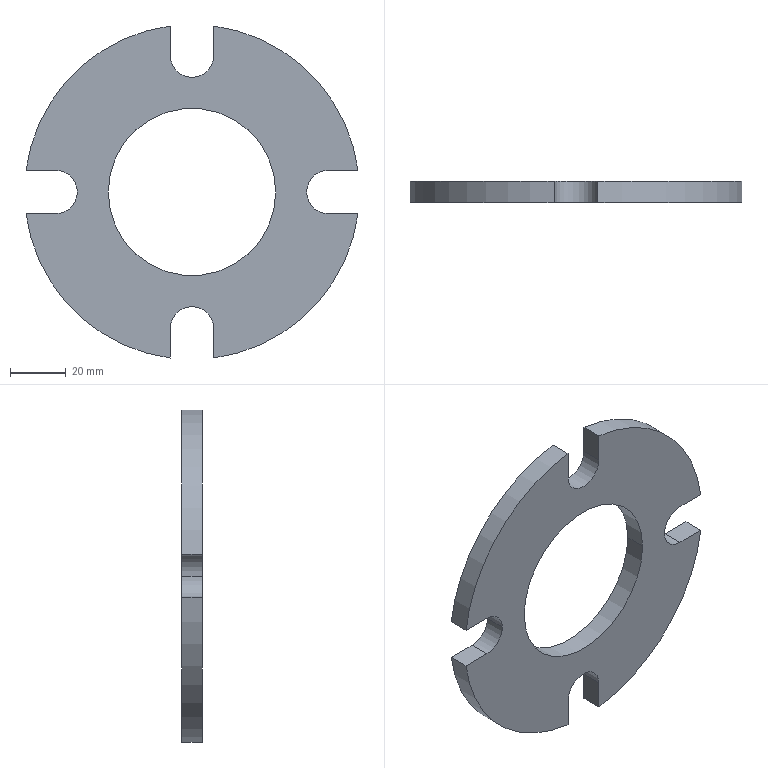Part | STEP file | Scale factor 1[14] | 1 solid | 22 faces | box 118.982 x 7.5 x 118.982 mm | volume 55635 mm3 | cylinder 12 | plane 10 | commonest cylinder face diameters 15.6 x6 120 x4 60 x2
STEP:
#1=CARTESIAN_POINT('',(-707.638,-288.773,3238.5));
#2=VERTEX_POINT('',#1);
#3=CARTESIAN_POINT('',(-699.838,-288.773,3246.3));
#4=VERTEX_POINT('',#3);
#5=CARTESIAN_POINT('',(-699.838,-288.773,3238.5));
#6=DIRECTION('',(0.,1.,0.));
#7=DIRECTION('',(1.,0.,0.000000001));
#8=AXIS2_PLACEMENT_3D('',#5,#6,#7);
#9=CIRCLE('',#8,7.8);
#10=EDGE_CURVE('',#2,#4,#9,.T.);
#11=ORIENTED_EDGE('',*,*,#10,.F.);
#12=CARTESIAN_POINT('',(-707.638,-281.273,3238.5));
#13=VERTEX_POINT('',#12);
#14=CARTESIAN_POINT('',(-707.638,-288.773,3238.5));
#15=DIRECTION('',(0.,1.,0.));
#16=VECTOR('',#15,1000.);
#17=LINE('',#14,#16);
#18=EDGE_CURVE('',#2,#13,#17,.T.);
#19=ORIENTED_EDGE('',*,*,#18,.T.);
#20=CARTESIAN_POINT('',(-699.838,-281.273,3246.3));
#21=VERTEX_POINT('',#20);
#22=CARTESIAN_POINT('',(-699.838,-281.273,3238.5));
#23=DIRECTION('',(0.,1.,0.));
#24=DIRECTION('',(1.,0.,0.000000001));
#25=AXIS2_PLACEMENT_3D('',#22,#23,#24);
#26=CIRCLE('',#25,7.8);
#27=EDGE_CURVE('',#13,#21,#26,.T.);
#28=ORIENTED_EDGE('',*,*,#27,.T.);
#29=CARTESIAN_POINT('',(-699.838,-288.773,3246.3));
#30=DIRECTION('',(0.,1.,0.));
#31=VECTOR('',#30,1000.);
#32=LINE('',#29,#31);
#33=EDGE_CURVE('',#4,#21,#32,.T.);
#34=ORIENTED_EDGE('',*,*,#33,.F.);
#35=EDGE_LOOP('',(#11,#19,#28,#34));
#36=FACE_OUTER_BOUND('',#35,.T.);
#37=CARTESIAN_POINT('',(-699.838,-288.773,3238.5));
#38=DIRECTION('',(0.,1.,0.));
#39=DIRECTION('',(-1.,0.,-0.000000001));
#40=AXIS2_PLACEMENT_3D('',#37,#38,#39);
#41=CYLINDRICAL_SURFACE('',#40,7.8);
#42=ADVANCED_FACE('',(#36),#41,.F.);
#43=CARTESIAN_POINT('',(-718.738,-281.273,3238.5));
#44=VERTEX_POINT('',#43);
#45=CARTESIAN_POINT('',(-778.738,-281.273,3238.5));
#46=VERTEX_POINT('',#45);
#47=CARTESIAN_POINT('',(-748.738,-281.273,3238.5));
#48=DIRECTION('',(0.,-1.,0.));
#49=DIRECTION('',(-1.,0.,-0.000000001));
#50=AXIS2_PLACEMENT_3D('',#47,#48,#49);
#51=CIRCLE('',#50,30.);
#52=EDGE_CURVE('',#44,#46,#51,.T.);
#53=ORIENTED_EDGE('',*,*,#52,.F.);
#54=CARTESIAN_POINT('',(-718.738,-288.773,3238.5));
#55=VERTEX_POINT('',#54);
#56=CARTESIAN_POINT('',(-718.738,-281.273,3238.5));
#57=DIRECTION('',(0.,1.,0.));
#58=VECTOR('',#57,1000.);
#59=LINE('',#56,#58);
#60=EDGE_CURVE('',#55,#44,#59,.T.);
#61=ORIENTED_EDGE('',*,*,#60,.F.);
#62=CARTESIAN_POINT('',(-778.738,-288.773,3238.5));
#63=VERTEX_POINT('',#62);
#64=CARTESIAN_POINT('',(-748.738,-288.773,3238.5));
#65=DIRECTION('',(0.,-1.,0.));
#66=DIRECTION('',(-1.,0.,-0.000000001));
#67=AXIS2_PLACEMENT_3D('',#64,#65,#66);
#68=CIRCLE('',#67,30.);
#69=EDGE_CURVE('',#55,#63,#68,.T.);
#70=ORIENTED_EDGE('',*,*,#69,.T.);
#71=CARTESIAN_POINT('',(-778.738,-281.273,3238.5));
#72=DIRECTION('',(0.,1.,0.));
#73=VECTOR('',#72,1000.);
#74=LINE('',#71,#73);
#75=EDGE_CURVE('',#63,#46,#74,.T.);
#76=ORIENTED_EDGE('',*,*,#75,.T.);
#77=EDGE_LOOP('',(#53,#61,#70,#76));
#78=FACE_OUTER_BOUND('',#77,.T.);
#79=CARTESIAN_POINT('',(-748.738,-281.273,3238.5));
#80=DIRECTION('',(0.,-1.,0.));
#81=DIRECTION('',(1.,0.,0.000000001));
#82=AXIS2_PLACEMENT_3D('',#79,#80,#81);
#83=CYLINDRICAL_SURFACE('',#82,30.);
#84=ADVANCED_FACE('',(#78),#83,.F.);
#85=CARTESIAN_POINT('',(-789.838,-288.773,3238.5));
#86=VERTEX_POINT('',#85);
#87=CARTESIAN_POINT('',(-797.638,-288.773,3230.7));
#88=VERTEX_POINT('',#87);
#89=CARTESIAN_POINT('',(-797.638,-288.773,3238.5));
#90=DIRECTION('',(0.,1.,0.));
#91=DIRECTION('',(1.,0.,0.000000001));
#92=AXIS2_PLACEMENT_3D('',#89,#90,#91);
#93=CIRCLE('',#92,7.8);
#94=EDGE_CURVE('',#86,#88,#93,.T.);
#95=ORIENTED_EDGE('',*,*,#94,.F.);
#96=CARTESIAN_POINT('',(-789.838,-281.273,3238.5));
#97=VERTEX_POINT('',#96);
#98=CARTESIAN_POINT('',(-789.838,-288.773,3238.5));
#99=DIRECTION('',(0.,1.,0.));
#100=VECTOR('',#99,1000.);
#101=LINE('',#98,#100);
#102=EDGE_CURVE('',#86,#97,#101,.T.);
#103=ORIENTED_EDGE('',*,*,#102,.T.);
#104=CARTESIAN_POINT('',(-797.638,-281.273,3230.7));
#105=VERTEX_POINT('',#104);
#106=CARTESIAN_POINT('',(-797.638,-281.273,3238.5));
#107=DIRECTION('',(0.,1.,0.));
#108=DIRECTION('',(1.,0.,0.000000001));
#109=AXIS2_PLACEMENT_3D('',#106,#107,#108);
#110=CIRCLE('',#109,7.8);
#111=EDGE_CURVE('',#97,#105,#110,.T.);
#112=ORIENTED_EDGE('',*,*,#111,.T.);
#113=CARTESIAN_POINT('',(-797.638,-288.773,3230.7));
#114=DIRECTION('',(0.,1.,0.));
#115=VECTOR('',#114,1000.);
#116=LINE('',#113,#115);
#117=EDGE_CURVE('',#88,#105,#116,.T.);
#118=ORIENTED_EDGE('',*,*,#117,.F.);
#119=EDGE_LOOP('',(#95,#103,#112,#118));
#120=FACE_OUTER_BOUND('',#119,.T.);
#121=CARTESIAN_POINT('',(-797.638,-288.773,3238.5));
#122=DIRECTION('',(0.,1.,0.));
#123=DIRECTION('',(-1.,0.,-0.000000001));
#124=AXIS2_PLACEMENT_3D('',#121,#122,#123);
#125=CYLINDRICAL_SURFACE('',#124,7.8);
#126=ADVANCED_FACE('',(#120),#125,.F.);
#127=CARTESIAN_POINT('',(-808.229,-288.773,3246.3));
#128=VERTEX_POINT('',#127);
#129=CARTESIAN_POINT('',(-808.229,-281.273,3246.3));
#130=VERTEX_POINT('',#129);
#131=CARTESIAN_POINT('',(-808.229,-288.773,3246.3));
#132=DIRECTION('',(0.,1.,0.));
#133=VECTOR('',#132,1000.);
#134=LINE('',#131,#133);
#135=EDGE_CURVE('',#128,#130,#134,.T.);
#136=ORIENTED_EDGE('',*,*,#135,.F.);
#137=CARTESIAN_POINT('',(-756.538,-288.773,3297.991));
#138=VERTEX_POINT('',#137);
#139=CARTESIAN_POINT('',(-748.738,-288.773,3238.5));
#140=DIRECTION('',(0.,1.,0.));
#141=DIRECTION('',(1.,0.,0.000000001));
#142=AXIS2_PLACEMENT_3D('',#139,#140,#141);
#143=CIRCLE('',#142,60.);
#144=EDGE_CURVE('',#128,#138,#143,.T.);
#145=ORIENTED_EDGE('',*,*,#144,.T.);
#146=CARTESIAN_POINT('',(-756.538,-281.273,3297.991));
#147=VERTEX_POINT('',#146);
#148=CARTESIAN_POINT('',(-756.538,-288.773,3297.991));
#149=DIRECTION('',(0.,1.,0.));
#150=VECTOR('',#149,1000.);
#151=LINE('',#148,#150);
#152=EDGE_CURVE('',#138,#147,#151,.T.);
#153=ORIENTED_EDGE('',*,*,#152,.T.);
#154=CARTESIAN_POINT('',(-748.738,-281.273,3238.5));
#155=DIRECTION('',(0.,1.,0.));
#156=DIRECTION('',(1.,0.,0.000000001));
#157=AXIS2_PLACEMENT_3D('',#154,#155,#156);
#158=CIRCLE('',#157,60.);
#159=EDGE_CURVE('',#130,#147,#158,.T.);
#160=ORIENTED_EDGE('',*,*,#159,.F.);
#161=EDGE_LOOP('',(#136,#145,#153,#160));
#162=FACE_OUTER_BOUND('',#161,.T.);
#163=CARTESIAN_POINT('',(-748.738,-281.273,3238.5));
#164=DIRECTION('',(0.,-1.,0.));
#165=DIRECTION('',(1.,0.,0.000000001));
#166=AXIS2_PLACEMENT_3D('',#163,#164,#165);
#167=CYLINDRICAL_SURFACE('',#166,60.);
#168=ADVANCED_FACE('',(#162),#167,.T.);
#169=CARTESIAN_POINT('',(-740.938,-288.773,3297.991));
#170=VERTEX_POINT('',#169);
#171=CARTESIAN_POINT('',(-740.938,-281.273,3297.991));
#172=VERTEX_POINT('',#171);
#173=CARTESIAN_POINT('',(-740.938,-288.773,3297.991));
#174=DIRECTION('',(0.,1.,0.));
#175=VECTOR('',#174,1000.);
#176=LINE('',#173,#175);
#177=EDGE_CURVE('',#170,#172,#176,.T.);
#178=ORIENTED_EDGE('',*,*,#177,.F.);
#179=CARTESIAN_POINT('',(-689.247,-288.773,3246.3));
#180=VERTEX_POINT('',#179);
#181=CARTESIAN_POINT('',(-748.738,-288.773,3238.5));
#182=DIRECTION('',(0.,1.,0.));
#183=DIRECTION('',(1.,0.,0.000000001));
#184=AXIS2_PLACEMENT_3D('',#181,#182,#183);
#185=CIRCLE('',#184,60.);
#186=EDGE_CURVE('',#170,#180,#185,.T.);
#187=ORIENTED_EDGE('',*,*,#186,.T.);
#188=CARTESIAN_POINT('',(-689.247,-281.273,3246.3));
#189=VERTEX_POINT('',#188);
#190=CARTESIAN_POINT('',(-689.247,-288.773,3246.3));
#191=DIRECTION('',(0.,1.,0.));
#192=VECTOR('',#191,1000.);
#193=LINE('',#190,#192);
#194=EDGE_CURVE('',#180,#189,#193,.T.);
#195=ORIENTED_EDGE('',*,*,#194,.T.);
#196=CARTESIAN_POINT('',(-748.738,-281.273,3238.5));
#197=DIRECTION('',(0.,1.,0.));
#198=DIRECTION('',(1.,0.,0.000000001));
#199=AXIS2_PLACEMENT_3D('',#196,#197,#198);
#200=CIRCLE('',#199,60.);
#201=EDGE_CURVE('',#172,#189,#200,.T.);
#202=ORIENTED_EDGE('',*,*,#201,.F.);
#203=EDGE_LOOP('',(#178,#187,#195,#202));
#204=FACE_OUTER_BOUND('',#203,.T.);
#205=CARTESIAN_POINT('',(-748.738,-281.273,3238.5));
#206=DIRECTION('',(0.,-1.,0.));
#207=DIRECTION('',(1.,0.,0.000000001));
#208=AXIS2_PLACEMENT_3D('',#205,#206,#207);
#209=CYLINDRICAL_SURFACE('',#208,60.);
#210=ADVANCED_FACE('',(#204),#209,.T.);
#211=CARTESIAN_POINT('',(-689.247,-288.773,3230.7));
#212=VERTEX_POINT('',#211);
#213=CARTESIAN_POINT('',(-689.247,-281.273,3230.7));
#214=VERTEX_POINT('',#213);
#215=CARTESIAN_POINT('',(-689.247,-288.773,3230.7));
#216=DIRECTION('',(0.,1.,0.));
#217=VECTOR('',#216,1000.);
#218=LINE('',#215,#217);
#219=EDGE_CURVE('',#212,#214,#218,.T.);
#220=ORIENTED_EDGE('',*,*,#219,.F.);
#221=CARTESIAN_POINT('',(-740.938,-288.773,3179.009));
#222=VERTEX_POINT('',#221);
#223=CARTESIAN_POINT('',(-748.738,-288.773,3238.5));
#224=DIRECTION('',(0.,1.,0.));
#225=DIRECTION('',(1.,0.,0.000000001));
#226=AXIS2_PLACEMENT_3D('',#223,#224,#225);
#227=CIRCLE('',#226,60.);
#228=EDGE_CURVE('',#212,#222,#227,.T.);
#229=ORIENTED_EDGE('',*,*,#228,.T.);
#230=CARTESIAN_POINT('',(-740.938,-281.273,3179.009));
#231=VERTEX_POINT('',#230);
#232=CARTESIAN_POINT('',(-740.938,-288.773,3179.009));
#233=DIRECTION('',(0.,1.,0.));
#234=VECTOR('',#233,1000.);
#235=LINE('',#232,#234);
#236=EDGE_CURVE('',#222,#231,#235,.T.);
#237=ORIENTED_EDGE('',*,*,#236,.T.);
#238=CARTESIAN_POINT('',(-748.738,-281.273,3238.5));
#239=DIRECTION('',(0.,1.,0.));
#240=DIRECTION('',(1.,0.,0.000000001));
#241=AXIS2_PLACEMENT_3D('',#238,#239,#240);
#242=CIRCLE('',#241,60.);
#243=EDGE_CURVE('',#214,#231,#242,.T.);
#244=ORIENTED_EDGE('',*,*,#243,.F.);
#245=EDGE_LOOP('',(#220,#229,#237,#244));
#246=FACE_OUTER_BOUND('',#245,.T.);
#247=CARTESIAN_POINT('',(-748.738,-281.273,3238.5));
#248=DIRECTION('',(0.,-1.,0.));
#249=DIRECTION('',(1.,0.,0.000000001));
#250=AXIS2_PLACEMENT_3D('',#247,#248,#249);
#251=CYLINDRICAL_SURFACE('',#250,60.);
#252=ADVANCED_FACE('',(#246),#251,.T.);
#253=CARTESIAN_POINT('',(-748.738,-281.273,3238.5));
#254=DIRECTION('',(0.,-1.,0.));
#255=DIRECTION('',(-1.,0.,-0.000000001));
#256=AXIS2_PLACEMENT_3D('',#253,#254,#255);
#257=CIRCLE('',#256,30.);
#258=EDGE_CURVE('',#46,#44,#257,.T.);
#259=ORIENTED_EDGE('',*,*,#258,.T.);
#260=ORIENTED_EDGE('',*,*,#52,.T.);
#261=EDGE_LOOP('',(#259,#260));
#262=FACE_BOUND('',#261,.T.);
#263=CARTESIAN_POINT('',(-797.638,-281.273,3246.3));
#264=VERTEX_POINT('',#263);
#265=CARTESIAN_POINT('',(-797.638,-281.273,3238.5));
#266=DIRECTION('',(0.,1.,0.));
#267=DIRECTION('',(1.,0.,0.000000001));
#268=AXIS2_PLACEMENT_3D('',#265,#266,#267);
#269=CIRCLE('',#268,7.8);
#270=EDGE_CURVE('',#264,#97,#269,.T.);
#271=ORIENTED_EDGE('',*,*,#270,.F.);
#272=CARTESIAN_POINT('',(-748.738,-281.273,3246.3));
#273=DIRECTION('',(-1.,0.,-0.000000001));
#274=VECTOR('',#273,1000.);
#275=LINE('',#272,#274);
#276=EDGE_CURVE('',#264,#130,#275,.T.);
#277=ORIENTED_EDGE('',*,*,#276,.T.);
#278=ORIENTED_EDGE('',*,*,#159,.T.);
#279=CARTESIAN_POINT('',(-756.538,-281.273,3287.4));
#280=VERTEX_POINT('',#279);
#281=CARTESIAN_POINT('',(-756.538,-281.273,3238.5));
#282=DIRECTION('',(-0.000000001,0.,1.));
#283=VECTOR('',#282,1000.);
#284=LINE('',#281,#283);
#285=EDGE_CURVE('',#280,#147,#284,.T.);
#286=ORIENTED_EDGE('',*,*,#285,.F.);
#287=CARTESIAN_POINT('',(-740.938,-281.273,3287.4));
#288=VERTEX_POINT('',#287);
#289=CARTESIAN_POINT('',(-748.738,-281.273,3287.4));
#290=DIRECTION('',(0.,1.,0.));
#291=DIRECTION('',(1.,0.,0.000000001));
#292=AXIS2_PLACEMENT_3D('',#289,#290,#291);
#293=CIRCLE('',#292,7.8);
#294=EDGE_CURVE('',#288,#280,#293,.T.);
#295=ORIENTED_EDGE('',*,*,#294,.F.);
#296=CARTESIAN_POINT('',(-740.938,-281.273,3238.5));
#297=DIRECTION('',(-0.000000001,0.,1.));
#298=VECTOR('',#297,1000.);
#299=LINE('',#296,#298);
#300=EDGE_CURVE('',#288,#172,#299,.T.);
#301=ORIENTED_EDGE('',*,*,#300,.T.);
#302=ORIENTED_EDGE('',*,*,#201,.T.);
#303=CARTESIAN_POINT('',(-748.738,-281.273,3246.3));
#304=DIRECTION('',(1.,0.,0.000000001));
#305=VECTOR('',#304,1000.);
#306=LINE('',#303,#305);
#307=EDGE_CURVE('',#21,#189,#306,.T.);
#308=ORIENTED_EDGE('',*,*,#307,.F.);
#309=ORIENTED_EDGE('',*,*,#27,.F.);
#310=CARTESIAN_POINT('',(-699.838,-281.273,3230.7));
#311=VERTEX_POINT('',#310);
#312=CARTESIAN_POINT('',(-699.838,-281.273,3238.5));
#313=DIRECTION('',(0.,1.,0.));
#314=DIRECTION('',(1.,0.,0.000000001));
#315=AXIS2_PLACEMENT_3D('',#312,#313,#314);
#316=CIRCLE('',#315,7.8);
#317=EDGE_CURVE('',#311,#13,#316,.T.);
#318=ORIENTED_EDGE('',*,*,#317,.F.);
#319=CARTESIAN_POINT('',(-748.738,-281.273,3230.7));
#320=DIRECTION('',(1.,0.,0.000000001));
#321=VECTOR('',#320,1000.);
#322=LINE('',#319,#321);
#323=EDGE_CURVE('',#311,#214,#322,.T.);
#324=ORIENTED_EDGE('',*,*,#323,.T.);
#325=ORIENTED_EDGE('',*,*,#243,.T.);
#326=CARTESIAN_POINT('',(-740.938,-281.273,3189.6));
#327=VERTEX_POINT('',#326);
#328=CARTESIAN_POINT('',(-740.938,-281.273,3238.5));
#329=DIRECTION('',(0.000000001,0.,-1.));
#330=VECTOR('',#329,1000.);
#331=LINE('',#328,#330);
#332=EDGE_CURVE('',#327,#231,#331,.T.);
#333=ORIENTED_EDGE('',*,*,#332,.F.);
#334=CARTESIAN_POINT('',(-756.538,-281.273,3189.6));
#335=VERTEX_POINT('',#334);
#336=CARTESIAN_POINT('',(-748.738,-281.273,3189.6));
#337=DIRECTION('',(0.,1.,0.));
#338=DIRECTION('',(1.,0.,0.000000001));
#339=AXIS2_PLACEMENT_3D('',#336,#337,#338);
#340=CIRCLE('',#339,7.8);
#341=EDGE_CURVE('',#335,#327,#340,.T.);
#342=ORIENTED_EDGE('',*,*,#341,.F.);
#343=CARTESIAN_POINT('',(-756.538,-281.273,3179.009));
#344=VERTEX_POINT('',#343);
#345=CARTESIAN_POINT('',(-756.538,-281.273,3238.5));
#346=DIRECTION('',(0.000000001,0.,-1.));
#347=VECTOR('',#346,1000.);
#348=LINE('',#345,#347);
#349=EDGE_CURVE('',#335,#344,#348,.T.);
#350=ORIENTED_EDGE('',*,*,#349,.T.);
#351=CARTESIAN_POINT('',(-808.229,-281.273,3230.7));
#352=VERTEX_POINT('',#351);
#353=CARTESIAN_POINT('',(-748.738,-281.273,3238.5));
#354=DIRECTION('',(0.,1.,0.));
#355=DIRECTION('',(1.,0.,0.000000001));
#356=AXIS2_PLACEMENT_3D('',#353,#354,#355);
#357=CIRCLE('',#356,60.);
#358=EDGE_CURVE('',#344,#352,#357,.T.);
#359=ORIENTED_EDGE('',*,*,#358,.T.);
#360=CARTESIAN_POINT('',(-748.738,-281.273,3230.7));
#361=DIRECTION('',(-1.,0.,-0.000000001));
#362=VECTOR('',#361,1000.);
#363=LINE('',#360,#362);
#364=EDGE_CURVE('',#105,#352,#363,.T.);
#365=ORIENTED_EDGE('',*,*,#364,.F.);
#366=ORIENTED_EDGE('',*,*,#111,.F.);
#367=EDGE_LOOP('',(#271,#277,#278,#286,#295,#301,#302,#308,#309,#318,#324,#325,#333,#342,#350,#359,#365,#366));
#368=FACE_OUTER_BOUND('',#367,.T.);
#369=CARTESIAN_POINT('',(-748.738,-281.273,3238.5));
#370=DIRECTION('',(0.,1.,0.));
#371=DIRECTION('',(-1.,0.,-0.000000001));
#372=AXIS2_PLACEMENT_3D('',#369,#370,#371);
#373=PLANE('',#372);
#374=ADVANCED_FACE('',(#262,#368),#373,.T.);
#375=CARTESIAN_POINT('',(-748.738,-288.773,3238.5));
#376=DIRECTION('',(0.,-1.,0.));
#377=DIRECTION('',(-1.,0.,-0.000000001));
#378=AXIS2_PLACEMENT_3D('',#375,#376,#377);
#379=CIRCLE('',#378,30.);
#380=EDGE_CURVE('',#63,#55,#379,.T.);
#381=ORIENTED_EDGE('',*,*,#380,.F.);
#382=ORIENTED_EDGE('',*,*,#69,.F.);
#383=EDGE_LOOP('',(#381,#382));
#384=FACE_BOUND('',#383,.T.);
#385=CARTESIAN_POINT('',(-797.638,-288.773,3246.3));
#386=VERTEX_POINT('',#385);
#387=CARTESIAN_POINT('',(-748.738,-288.773,3246.3));
#388=DIRECTION('',(-1.,0.,-0.000000001));
#389=VECTOR('',#388,1000.);
#390=LINE('',#387,#389);
#391=EDGE_CURVE('',#386,#128,#390,.T.);
#392=ORIENTED_EDGE('',*,*,#391,.F.);
#393=CARTESIAN_POINT('',(-797.638,-288.773,3238.5));
#394=DIRECTION('',(0.,1.,0.));
#395=DIRECTION('',(1.,0.,0.000000001));
#396=AXIS2_PLACEMENT_3D('',#393,#394,#395);
#397=CIRCLE('',#396,7.8);
#398=EDGE_CURVE('',#386,#86,#397,.T.);
#399=ORIENTED_EDGE('',*,*,#398,.T.);
#400=ORIENTED_EDGE('',*,*,#94,.T.);
#401=CARTESIAN_POINT('',(-808.229,-288.773,3230.7));
#402=VERTEX_POINT('',#401);
#403=CARTESIAN_POINT('',(-748.738,-288.773,3230.7));
#404=DIRECTION('',(-1.,0.,-0.000000001));
#405=VECTOR('',#404,1000.);
#406=LINE('',#403,#405);
#407=EDGE_CURVE('',#88,#402,#406,.T.);
#408=ORIENTED_EDGE('',*,*,#407,.T.);
#409=CARTESIAN_POINT('',(-756.538,-288.773,3179.009));
#410=VERTEX_POINT('',#409);
#411=CARTESIAN_POINT('',(-748.738,-288.773,3238.5));
#412=DIRECTION('',(0.,1.,0.));
#413=DIRECTION('',(1.,0.,0.000000001));
#414=AXIS2_PLACEMENT_3D('',#411,#412,#413);
#415=CIRCLE('',#414,60.);
#416=EDGE_CURVE('',#410,#402,#415,.T.);
#417=ORIENTED_EDGE('',*,*,#416,.F.);
#418=CARTESIAN_POINT('',(-756.538,-288.773,3189.6));
#419=VERTEX_POINT('',#418);
#420=CARTESIAN_POINT('',(-756.538,-288.773,3238.5));
#421=DIRECTION('',(0.000000001,0.,-1.));
#422=VECTOR('',#421,1000.);
#423=LINE('',#420,#422);
#424=EDGE_CURVE('',#419,#410,#423,.T.);
#425=ORIENTED_EDGE('',*,*,#424,.F.);
#426=CARTESIAN_POINT('',(-740.938,-288.773,3189.6));
#427=VERTEX_POINT('',#426);
#428=CARTESIAN_POINT('',(-748.738,-288.773,3189.6));
#429=DIRECTION('',(0.,1.,0.));
#430=DIRECTION('',(1.,0.,0.000000001));
#431=AXIS2_PLACEMENT_3D('',#428,#429,#430);
#432=CIRCLE('',#431,7.8);
#433=EDGE_CURVE('',#419,#427,#432,.T.);
#434=ORIENTED_EDGE('',*,*,#433,.T.);
#435=CARTESIAN_POINT('',(-740.938,-288.773,3238.5));
#436=DIRECTION('',(0.000000001,0.,-1.));
#437=VECTOR('',#436,1000.);
#438=LINE('',#435,#437);
#439=EDGE_CURVE('',#427,#222,#438,.T.);
#440=ORIENTED_EDGE('',*,*,#439,.T.);
#441=ORIENTED_EDGE('',*,*,#228,.F.);
#442=CARTESIAN_POINT('',(-699.838,-288.773,3230.7));
#443=VERTEX_POINT('',#442);
#444=CARTESIAN_POINT('',(-748.738,-288.773,3230.7));
#445=DIRECTION('',(1.,0.,0.000000001));
#446=VECTOR('',#445,1000.);
#447=LINE('',#444,#446);
#448=EDGE_CURVE('',#443,#212,#447,.T.);
#449=ORIENTED_EDGE('',*,*,#448,.F.);
#450=CARTESIAN_POINT('',(-699.838,-288.773,3238.5));
#451=DIRECTION('',(0.,1.,0.));
#452=DIRECTION('',(1.,0.,0.000000001));
#453=AXIS2_PLACEMENT_3D('',#450,#451,#452);
#454=CIRCLE('',#453,7.8);
#455=EDGE_CURVE('',#443,#2,#454,.T.);
#456=ORIENTED_EDGE('',*,*,#455,.T.);
#457=ORIENTED_EDGE('',*,*,#10,.T.);
#458=CARTESIAN_POINT('',(-748.738,-288.773,3246.3));
#459=DIRECTION('',(1.,0.,0.000000001));
#460=VECTOR('',#459,1000.);
#461=LINE('',#458,#460);
#462=EDGE_CURVE('',#4,#180,#461,.T.);
#463=ORIENTED_EDGE('',*,*,#462,.T.);
#464=ORIENTED_EDGE('',*,*,#186,.F.);
#465=CARTESIAN_POINT('',(-740.938,-288.773,3287.4));
#466=VERTEX_POINT('',#465);
#467=CARTESIAN_POINT('',(-740.938,-288.773,3238.5));
#468=DIRECTION('',(-0.000000001,0.,1.));
#469=VECTOR('',#468,1000.);
#470=LINE('',#467,#469);
#471=EDGE_CURVE('',#466,#170,#470,.T.);
#472=ORIENTED_EDGE('',*,*,#471,.F.);
#473=CARTESIAN_POINT('',(-756.538,-288.773,3287.4));
#474=VERTEX_POINT('',#473);
#475=CARTESIAN_POINT('',(-748.738,-288.773,3287.4));
#476=DIRECTION('',(0.,1.,0.));
#477=DIRECTION('',(1.,0.,0.000000001));
#478=AXIS2_PLACEMENT_3D('',#475,#476,#477);
#479=CIRCLE('',#478,7.8);
#480=EDGE_CURVE('',#466,#474,#479,.T.);
#481=ORIENTED_EDGE('',*,*,#480,.T.);
#482=CARTESIAN_POINT('',(-756.538,-288.773,3238.5));
#483=DIRECTION('',(-0.000000001,0.,1.));
#484=VECTOR('',#483,1000.);
#485=LINE('',#482,#484);
#486=EDGE_CURVE('',#474,#138,#485,.T.);
#487=ORIENTED_EDGE('',*,*,#486,.T.);
#488=ORIENTED_EDGE('',*,*,#144,.F.);
#489=EDGE_LOOP('',(#392,#399,#400,#408,#417,#425,#434,#440,#441,#449,#456,#457,#463,#464,#472,#481,#487,#488));
#490=FACE_OUTER_BOUND('',#489,.T.);
#491=CARTESIAN_POINT('',(-748.738,-288.773,3238.5));
#492=DIRECTION('',(0.,1.,0.));
#493=DIRECTION('',(-1.,0.,-0.000000001));
#494=AXIS2_PLACEMENT_3D('',#491,#492,#493);
#495=PLANE('',#494);
#496=ADVANCED_FACE('',(#384,#490),#495,.F.);
#497=ORIENTED_EDGE('',*,*,#416,.T.);
#498=CARTESIAN_POINT('',(-808.229,-288.773,3230.7));
#499=DIRECTION('',(0.,1.,0.));
#500=VECTOR('',#499,1000.);
#501=LINE('',#498,#500);
#502=EDGE_CURVE('',#402,#352,#501,.T.);
#503=ORIENTED_EDGE('',*,*,#502,.T.);
#504=ORIENTED_EDGE('',*,*,#358,.F.);
#505=CARTESIAN_POINT('',(-756.538,-288.773,3179.009));
#506=DIRECTION('',(0.,1.,0.));
#507=VECTOR('',#506,1000.);
#508=LINE('',#505,#507);
#509=EDGE_CURVE('',#410,#344,#508,.T.);
#510=ORIENTED_EDGE('',*,*,#509,.F.);
#511=EDGE_LOOP('',(#497,#503,#504,#510));
#512=FACE_OUTER_BOUND('',#511,.T.);
#513=CARTESIAN_POINT('',(-748.738,-281.273,3238.5));
#514=DIRECTION('',(0.,-1.,0.));
#515=DIRECTION('',(1.,0.,0.000000001));
#516=AXIS2_PLACEMENT_3D('',#513,#514,#515);
#517=CYLINDRICAL_SURFACE('',#516,60.);
#518=ADVANCED_FACE('',(#512),#517,.T.);
#519=ORIENTED_EDGE('',*,*,#349,.F.);
#520=CARTESIAN_POINT('',(-756.538,-288.773,3189.6));
#521=DIRECTION('',(0.,1.,0.));
#522=VECTOR('',#521,1000.);
#523=LINE('',#520,#522);
#524=EDGE_CURVE('',#419,#335,#523,.T.);
#525=ORIENTED_EDGE('',*,*,#524,.F.);
#526=ORIENTED_EDGE('',*,*,#424,.T.);
#527=ORIENTED_EDGE('',*,*,#509,.T.);
#528=EDGE_LOOP('',(#519,#525,#526,#527));
#529=FACE_OUTER_BOUND('',#528,.T.);
#530=CARTESIAN_POINT('',(-756.538,-288.773,3238.5));
#531=DIRECTION('',(1.,0.,0.000000001));
#532=DIRECTION('',(-0.000000001,0.,1.));
#533=AXIS2_PLACEMENT_3D('',#530,#531,#532);
#534=PLANE('',#533);
#535=ADVANCED_FACE('',(#529),#534,.T.);
#536=ORIENTED_EDGE('',*,*,#332,.T.);
#537=ORIENTED_EDGE('',*,*,#236,.F.);
#538=ORIENTED_EDGE('',*,*,#439,.F.);
#539=CARTESIAN_POINT('',(-740.938,-288.773,3189.6));
#540=DIRECTION('',(0.,1.,0.));
#541=VECTOR('',#540,1000.);
#542=LINE('',#539,#541);
#543=EDGE_CURVE('',#427,#327,#542,.T.);
#544=ORIENTED_EDGE('',*,*,#543,.T.);
#545=EDGE_LOOP('',(#536,#537,#538,#544));
#546=FACE_OUTER_BOUND('',#545,.T.);
#547=CARTESIAN_POINT('',(-740.938,-288.773,3238.5));
#548=DIRECTION('',(1.,0.,0.000000001));
#549=DIRECTION('',(-0.000000001,0.,1.));
#550=AXIS2_PLACEMENT_3D('',#547,#548,#549);
#551=PLANE('',#550);
#552=ADVANCED_FACE('',(#546),#551,.F.);
#553=ORIENTED_EDGE('',*,*,#341,.T.);
#554=ORIENTED_EDGE('',*,*,#543,.F.);
#555=ORIENTED_EDGE('',*,*,#433,.F.);
#556=ORIENTED_EDGE('',*,*,#524,.T.);
#557=EDGE_LOOP('',(#553,#554,#555,#556));
#558=FACE_OUTER_BOUND('',#557,.T.);
#559=CARTESIAN_POINT('',(-748.738,-288.773,3189.6));
#560=DIRECTION('',(0.,1.,0.));
#561=DIRECTION('',(-1.,0.,-0.000000001));
#562=AXIS2_PLACEMENT_3D('',#559,#560,#561);
#563=CYLINDRICAL_SURFACE('',#562,7.8);
#564=ADVANCED_FACE('',(#558),#563,.F.);
#565=ORIENTED_EDGE('',*,*,#323,.F.);
#566=CARTESIAN_POINT('',(-699.838,-288.773,3230.7));
#567=DIRECTION('',(0.,1.,0.));
#568=VECTOR('',#567,1000.);
#569=LINE('',#566,#568);
#570=EDGE_CURVE('',#443,#311,#569,.T.);
#571=ORIENTED_EDGE('',*,*,#570,.F.);
#572=ORIENTED_EDGE('',*,*,#448,.T.);
#573=ORIENTED_EDGE('',*,*,#219,.T.);
#574=EDGE_LOOP('',(#565,#571,#572,#573));
#575=FACE_OUTER_BOUND('',#574,.T.);
#576=CARTESIAN_POINT('',(-748.738,-288.773,3230.7));
#577=DIRECTION('',(-0.000000001,0.,1.));
#578=DIRECTION('',(-1.,0.,-0.000000001));
#579=AXIS2_PLACEMENT_3D('',#576,#577,#578);
#580=PLANE('',#579);
#581=ADVANCED_FACE('',(#575),#580,.T.);
#582=ORIENTED_EDGE('',*,*,#307,.T.);
#583=ORIENTED_EDGE('',*,*,#194,.F.);
#584=ORIENTED_EDGE('',*,*,#462,.F.);
#585=ORIENTED_EDGE('',*,*,#33,.T.);
#586=EDGE_LOOP('',(#582,#583,#584,#585));
#587=FACE_OUTER_BOUND('',#586,.T.);
#588=CARTESIAN_POINT('',(-748.738,-288.773,3246.3));
#589=DIRECTION('',(-0.000000001,0.,1.));
#590=DIRECTION('',(-1.,0.,-0.000000001));
#591=AXIS2_PLACEMENT_3D('',#588,#589,#590);
#592=PLANE('',#591);
#593=ADVANCED_FACE('',(#587),#592,.F.);
#594=ORIENTED_EDGE('',*,*,#18,.F.);
#595=ORIENTED_EDGE('',*,*,#455,.F.);
#596=ORIENTED_EDGE('',*,*,#570,.T.);
#597=ORIENTED_EDGE('',*,*,#317,.T.);
#598=EDGE_LOOP('',(#594,#595,#596,#597));
#599=FACE_OUTER_BOUND('',#598,.T.);
#600=CARTESIAN_POINT('',(-699.838,-288.773,3238.5));
#601=DIRECTION('',(0.,1.,0.));
#602=DIRECTION('',(-1.,0.,-0.000000001));
#603=AXIS2_PLACEMENT_3D('',#600,#601,#602);
#604=CYLINDRICAL_SURFACE('',#603,7.8);
#605=ADVANCED_FACE('',(#599),#604,.F.);
#606=ORIENTED_EDGE('',*,*,#300,.F.);
#607=CARTESIAN_POINT('',(-740.938,-288.773,3287.4));
#608=DIRECTION('',(0.,1.,0.));
#609=VECTOR('',#608,1000.);
#610=LINE('',#607,#609);
#611=EDGE_CURVE('',#466,#288,#610,.T.);
#612=ORIENTED_EDGE('',*,*,#611,.F.);
#613=ORIENTED_EDGE('',*,*,#471,.T.);
#614=ORIENTED_EDGE('',*,*,#177,.T.);
#615=EDGE_LOOP('',(#606,#612,#613,#614));
#616=FACE_OUTER_BOUND('',#615,.T.);
#617=CARTESIAN_POINT('',(-740.938,-288.773,3238.5));
#618=DIRECTION('',(-1.,0.,-0.000000001));
#619=DIRECTION('',(0.,-1.,0.));
#620=AXIS2_PLACEMENT_3D('',#617,#618,#619);
#621=PLANE('',#620);
#622=ADVANCED_FACE('',(#616),#621,.T.);
#623=ORIENTED_EDGE('',*,*,#285,.T.);
#624=ORIENTED_EDGE('',*,*,#152,.F.);
#625=ORIENTED_EDGE('',*,*,#486,.F.);
#626=CARTESIAN_POINT('',(-756.538,-288.773,3287.4));
#627=DIRECTION('',(0.,1.,0.));
#628=VECTOR('',#627,1000.);
#629=LINE('',#626,#628);
#630=EDGE_CURVE('',#474,#280,#629,.T.);
#631=ORIENTED_EDGE('',*,*,#630,.T.);
#632=EDGE_LOOP('',(#623,#624,#625,#631));
#633=FACE_OUTER_BOUND('',#632,.T.);
#634=CARTESIAN_POINT('',(-756.538,-288.773,3238.5));
#635=DIRECTION('',(-1.,0.,-0.000000001));
#636=DIRECTION('',(0.,-1.,0.));
#637=AXIS2_PLACEMENT_3D('',#634,#635,#636);
#638=PLANE('',#637);
#639=ADVANCED_FACE('',(#633),#638,.F.);
#640=ORIENTED_EDGE('',*,*,#294,.T.);
#641=ORIENTED_EDGE('',*,*,#630,.F.);
#642=ORIENTED_EDGE('',*,*,#480,.F.);
#643=ORIENTED_EDGE('',*,*,#611,.T.);
#644=EDGE_LOOP('',(#640,#641,#642,#643));
#645=FACE_OUTER_BOUND('',#644,.T.);
#646=CARTESIAN_POINT('',(-748.738,-288.773,3287.4));
#647=DIRECTION('',(0.,1.,0.));
#648=DIRECTION('',(-1.,0.,-0.000000001));
#649=AXIS2_PLACEMENT_3D('',#646,#647,#648);
#650=CYLINDRICAL_SURFACE('',#649,7.8);
#651=ADVANCED_FACE('',(#645),#650,.F.);
#652=ORIENTED_EDGE('',*,*,#276,.F.);
#653=CARTESIAN_POINT('',(-797.638,-288.773,3246.3));
#654=DIRECTION('',(0.,1.,0.));
#655=VECTOR('',#654,1000.);
#656=LINE('',#653,#655);
#657=EDGE_CURVE('',#386,#264,#656,.T.);
#658=ORIENTED_EDGE('',*,*,#657,.F.);
#659=ORIENTED_EDGE('',*,*,#391,.T.);
#660=ORIENTED_EDGE('',*,*,#135,.T.);
#661=EDGE_LOOP('',(#652,#658,#659,#660));
#662=FACE_OUTER_BOUND('',#661,.T.);
#663=CARTESIAN_POINT('',(-748.738,-288.773,3246.3));
#664=DIRECTION('',(0.000000001,0.,-1.));
#665=DIRECTION('',(1.,0.,0.000000001));
#666=AXIS2_PLACEMENT_3D('',#663,#664,#665);
#667=PLANE('',#666);
#668=ADVANCED_FACE('',(#662),#667,.T.);
#669=ORIENTED_EDGE('',*,*,#364,.T.);
#670=ORIENTED_EDGE('',*,*,#502,.F.);
#671=ORIENTED_EDGE('',*,*,#407,.F.);
#672=ORIENTED_EDGE('',*,*,#117,.T.);
#673=EDGE_LOOP('',(#669,#670,#671,#672));
#674=FACE_OUTER_BOUND('',#673,.T.);
#675=CARTESIAN_POINT('',(-748.738,-288.773,3230.7));
#676=DIRECTION('',(0.000000001,0.,-1.));
#677=DIRECTION('',(1.,0.,0.000000001));
#678=AXIS2_PLACEMENT_3D('',#675,#676,#677);
#679=PLANE('',#678);
#680=ADVANCED_FACE('',(#674),#679,.F.);
#681=ORIENTED_EDGE('',*,*,#102,.F.);
#682=ORIENTED_EDGE('',*,*,#398,.F.);
#683=ORIENTED_EDGE('',*,*,#657,.T.);
#684=ORIENTED_EDGE('',*,*,#270,.T.);
#685=EDGE_LOOP('',(#681,#682,#683,#684));
#686=FACE_OUTER_BOUND('',#685,.T.);
#687=CARTESIAN_POINT('',(-797.638,-288.773,3238.5));
#688=DIRECTION('',(0.,1.,0.));
#689=DIRECTION('',(-1.,0.,-0.000000001));
#690=AXIS2_PLACEMENT_3D('',#687,#688,#689);
#691=CYLINDRICAL_SURFACE('',#690,7.8);
#692=ADVANCED_FACE('',(#686),#691,.F.);
#693=ORIENTED_EDGE('',*,*,#60,.T.);
#694=ORIENTED_EDGE('',*,*,#258,.F.);
#695=ORIENTED_EDGE('',*,*,#75,.F.);
#696=ORIENTED_EDGE('',*,*,#380,.T.);
#697=EDGE_LOOP('',(#693,#694,#695,#696));
#698=FACE_OUTER_BOUND('',#697,.T.);
#699=CARTESIAN_POINT('',(-748.738,-281.273,3238.5));
#700=DIRECTION('',(0.,-1.,0.));
#701=DIRECTION('',(1.,0.,0.000000001));
#702=AXIS2_PLACEMENT_3D('',#699,#700,#701);
#703=CYLINDRICAL_SURFACE('',#702,30.);
#704=ADVANCED_FACE('',(#698),#703,.F.);
#705=CLOSED_SHELL('',(#42,#84,#126,#168,#210,#252,#374,#496,#518,#535,#552,#564,#581,#593,#605,#622,#639,#651,#668,#680,#692,#704));
#706=MANIFOLD_SOLID_BREP('',#705);
#707=CARTESIAN_POINT('',(0.,0.,0.));
#708=DIRECTION('',(0.,0.,1.));
#709=DIRECTION('',(1.,0.,0.));
#710=AXIS2_PLACEMENT_3D('',#707,#708,#709);
#711=(LENGTH_UNIT()NAMED_UNIT(*)SI_UNIT(.MILLI.,.METRE.));
#712=UNCERTAINTY_MEASURE_WITH_UNIT(LENGTH_MEASURE(0.00001),#711,'','');
#713=(NAMED_UNIT(*)PLANE_ANGLE_UNIT()SI_UNIT($,.RADIAN.));
#714=(NAMED_UNIT(*)SI_UNIT($,.STERADIAN.)SOLID_ANGLE_UNIT());
#715=(GEOMETRIC_REPRESENTATION_CONTEXT(3)GLOBAL_UNCERTAINTY_ASSIGNED_CONTEXT((#712))GLOBAL_UNIT_ASSIGNED_CONTEXT((#711,#713,#714))REPRESENTATION_CONTEXT('',''));
#716=ADVANCED_BREP_SHAPE_REPRESENTATION('',(#706,#710),#715);